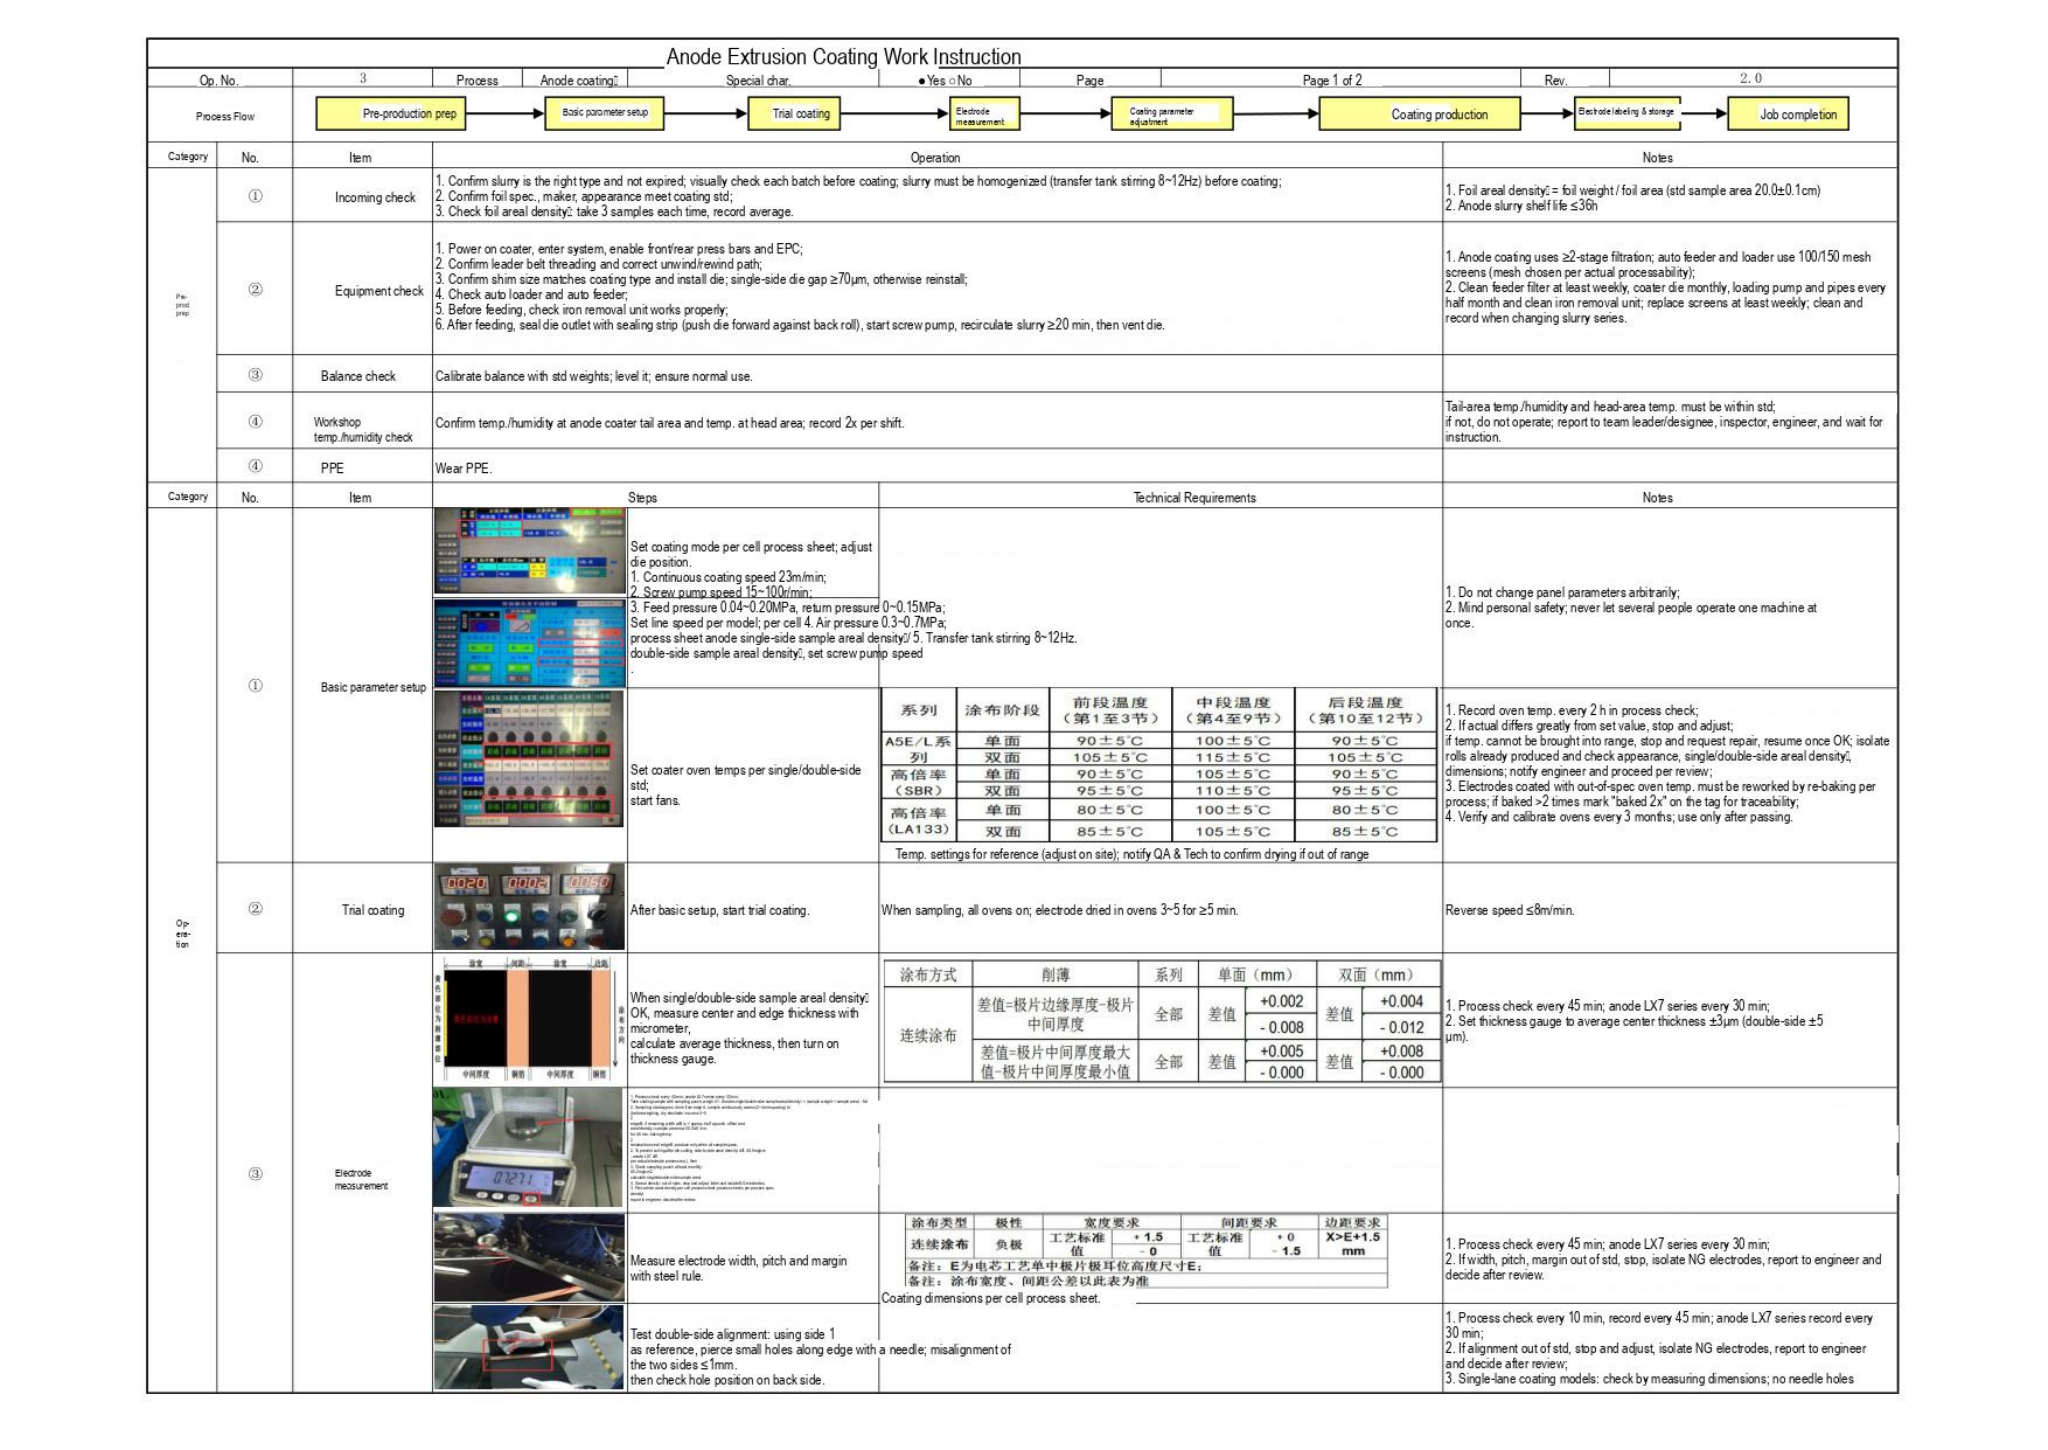Anode Extrusion Coating Work Instruction

| Op. No. | 3 | Process | Anode coating | Special char. | ●Yes ○No | Page | Page 1 of 2 | Rev. | 2.0 |
|---|---|---|---|---|---|---|---|---|---|

Process Flow: Pre-production prep → Basic parameter setup → Trial coating → Electrode measurement → Coating parameter adjustment → Coating production → Electrode labeling & storage → Job completion

| Category | No. | Item | Operation | Notes |
|---|---|---|---|---|
| Pre-prod prep | ① | Incoming check | 1. Confirm slurry is the right type and not expired; visually check each batch before coating; slurry must be homogenized (transfer tank stirring 8~12Hz) before coating;<br>2. Confirm foil spec., maker, appearance meet coating std;<br>3. Check foil areal density: take 3 samples each time, record average. | 1. Foil areal density = foil weight / foil area (std sample area 20.0±0.1cm)<br>2. Anode slurry shelf life ≤36h |
| | ② | Equipment check | 1. Power on coater, enter system, enable front/rear press bars and EPC;<br>2. Confirm leader belt threading and correct unwind/rewind path;<br>3. Confirm shim size matches coating type and install die; single-side die gap ≥70μm, otherwise reinstall;<br>4. Check auto loader and auto feeder;<br>5. Before feeding, check iron removal unit works properly;<br>6. After feeding, seal die outlet with sealing strip (push die forward against back roll), start screw pump, recirculate slurry ≥20 min, then vent die. | 1. Anode coating uses ≥2-stage filtration; auto feeder and loader use 100/150 mesh screens (mesh chosen per actual processability);<br>2. Clean feeder filter at least weekly, coater die monthly, loading pump and pipes every half month and clean iron removal unit; replace screens at least weekly; clean and record when changing slurry series. |
| | ③ | Balance check | Calibrate balance with std weights; level it; ensure normal use. | |
| | ④ | Workshop temp./humidity check | Confirm temp./humidity at anode coater tail area and temp. at head area; record 2x per shift. | Tail-area temp./humidity and head-area temp. must be within std; if not, do not operate; report to team leader/designee, inspector, engineer, and wait for instruction. |
| | ④ | PPE | Wear PPE. | |

| Category | No. | Item | Steps | Technical Requirements | Notes |
|---|---|---|---|---|---|
| Operation | ① | Basic parameter setup | Set coating mode per cell process sheet; adjust die position.<br>1. Continuous coating speed 23m/min;<br>2. Screw pump speed 15~100r/min;<br>3. Feed pressure 0.04~0.20MPa, return pressure 0~0.15MPa;<br>Set line speed per model; per cell 4. Air pressure 0.3~0.7MPa;<br>process sheet anode single-side sample areal density/ 5. Transfer tank stirring 8~12Hz.<br>double-side sample areal density, set screw pump speed | | 1. Do not change panel parameters arbitrarily;<br>2. Mind personal safety; never let several people operate one machine at once. |
| | | | Set coater oven temps per single/double-side std;<br>start fans. | (see oven temperature table below)<br>Temp. settings for reference (adjust on site); notify QA & Tech to confirm drying if out of range | 1. Record oven temp. every 2 h in process check;<br>2. If actual differs greatly from set value, stop and adjust;<br>if temp. cannot be brought into range, stop and request repair, resume once OK; isolate rolls already produced and check appearance, single/double-side areal density, dimensions; notify engineer and proceed per review;<br>3. Electrodes coated with out-of-spec oven temp. must be reworked by re-baking per process; if baked >2 times mark "baked 2x" on the tag for traceability;<br>4. Verify and calibrate ovens every 3 months; use only after passing. |
| | ② | Trial coating | After basic setup, start trial coating. | When sampling, all ovens on; electrode dried in ovens 3~5 for ≥5 min. | Reverse speed ≤8m/min. |
| | ③ | Electrode measurement | When single/double-side sample areal density OK, measure center and edge thickness with micrometer,<br>calculate average thickness, then turn on thickness gauge. | (see thinning table below) | 1. Process check every 45 min; anode LX7 series every 30 min;<br>2. Set thickness gauge to average center thickness ±3μm (double-side ±5 μm). |
| | | | Measure electrode width, pitch and margin with steel rule. | (see dimension table below)<br>Coating dimensions per cell process sheet. | 1. Process check every 45 min; anode LX7 series every 30 min;<br>2. If width, pitch, margin out of std, stop, isolate NG electrodes, report to engineer and decide after review. |
| | | | Test double-side alignment: using side 1 as reference, pierce small holes along edge with a needle; misalignment of the two sides ≤1mm.<br>then check hole position on back side. | | 1. Process check every 10 min, record every 45 min; anode LX7 series record every 30 min;<br>2. If alignment out of std, stop and adjust, isolate NG electrodes, report to engineer and decide after review;<br>3. Single-lane coating models: check by measuring dimensions; no needle holes |

Oven temperature table:

| 系列 | 涂布阶段 | 前段温度（第1至3节） | 中段温度（第4至9节） | 后段温度（第10至12节） |
|---|---|---|---|---|
| A5E/L系列 | 单面 | 90±5℃ | 100±5℃ | 90±5℃ |
| | 双面 | 105±5℃ | 115±5℃ | 105±5℃ |
| 高倍率（SBR） | 单面 | 90±5℃ | 105±5℃ | 90±5℃ |
| | 双面 | 95±5℃ | 110±5℃ | 95±5℃ |
| 高倍率（LA133） | 单面 | 80±5℃ | 100±5℃ | 80±5℃ |
| | 双面 | 85±5℃ | 105±5℃ | 85±5℃ |

Thinning table:

| 涂布方式 | 削薄 | 系列 | 单面（mm） | | 双面（mm） | |
|---|---|---|---|---|---|---|
| 连续涂布 | 差值=极片边缘厚度-极片中间厚度 | 全部 | 差值 | +0.002 / -0.008 | 差值 | +0.004 / -0.012 |
| | 差值=极片中间厚度最大值-极片中间厚度最小值 | 全部 | 差值 | +0.005 / -0.000 | 差值 | +0.008 / -0.000 |

Dimension table:

| 涂布类型 | 极性 | 宽度要求 | | 间距要求 | | 边距要求 |
|---|---|---|---|---|---|---|
| 连续涂布 | 负极 | 工艺标准值 | +1.5 / -0 | 工艺标准值 | +0 / -1.5 | X>E+1.5 mm |

备注：E为电芯工艺单中极片极耳位高度尺寸E;
备注：涂布宽度、间距公差以此表为准

Words in photographs (thickness diagram): 中间厚度, 铜箔, 中间厚度, 铜箔
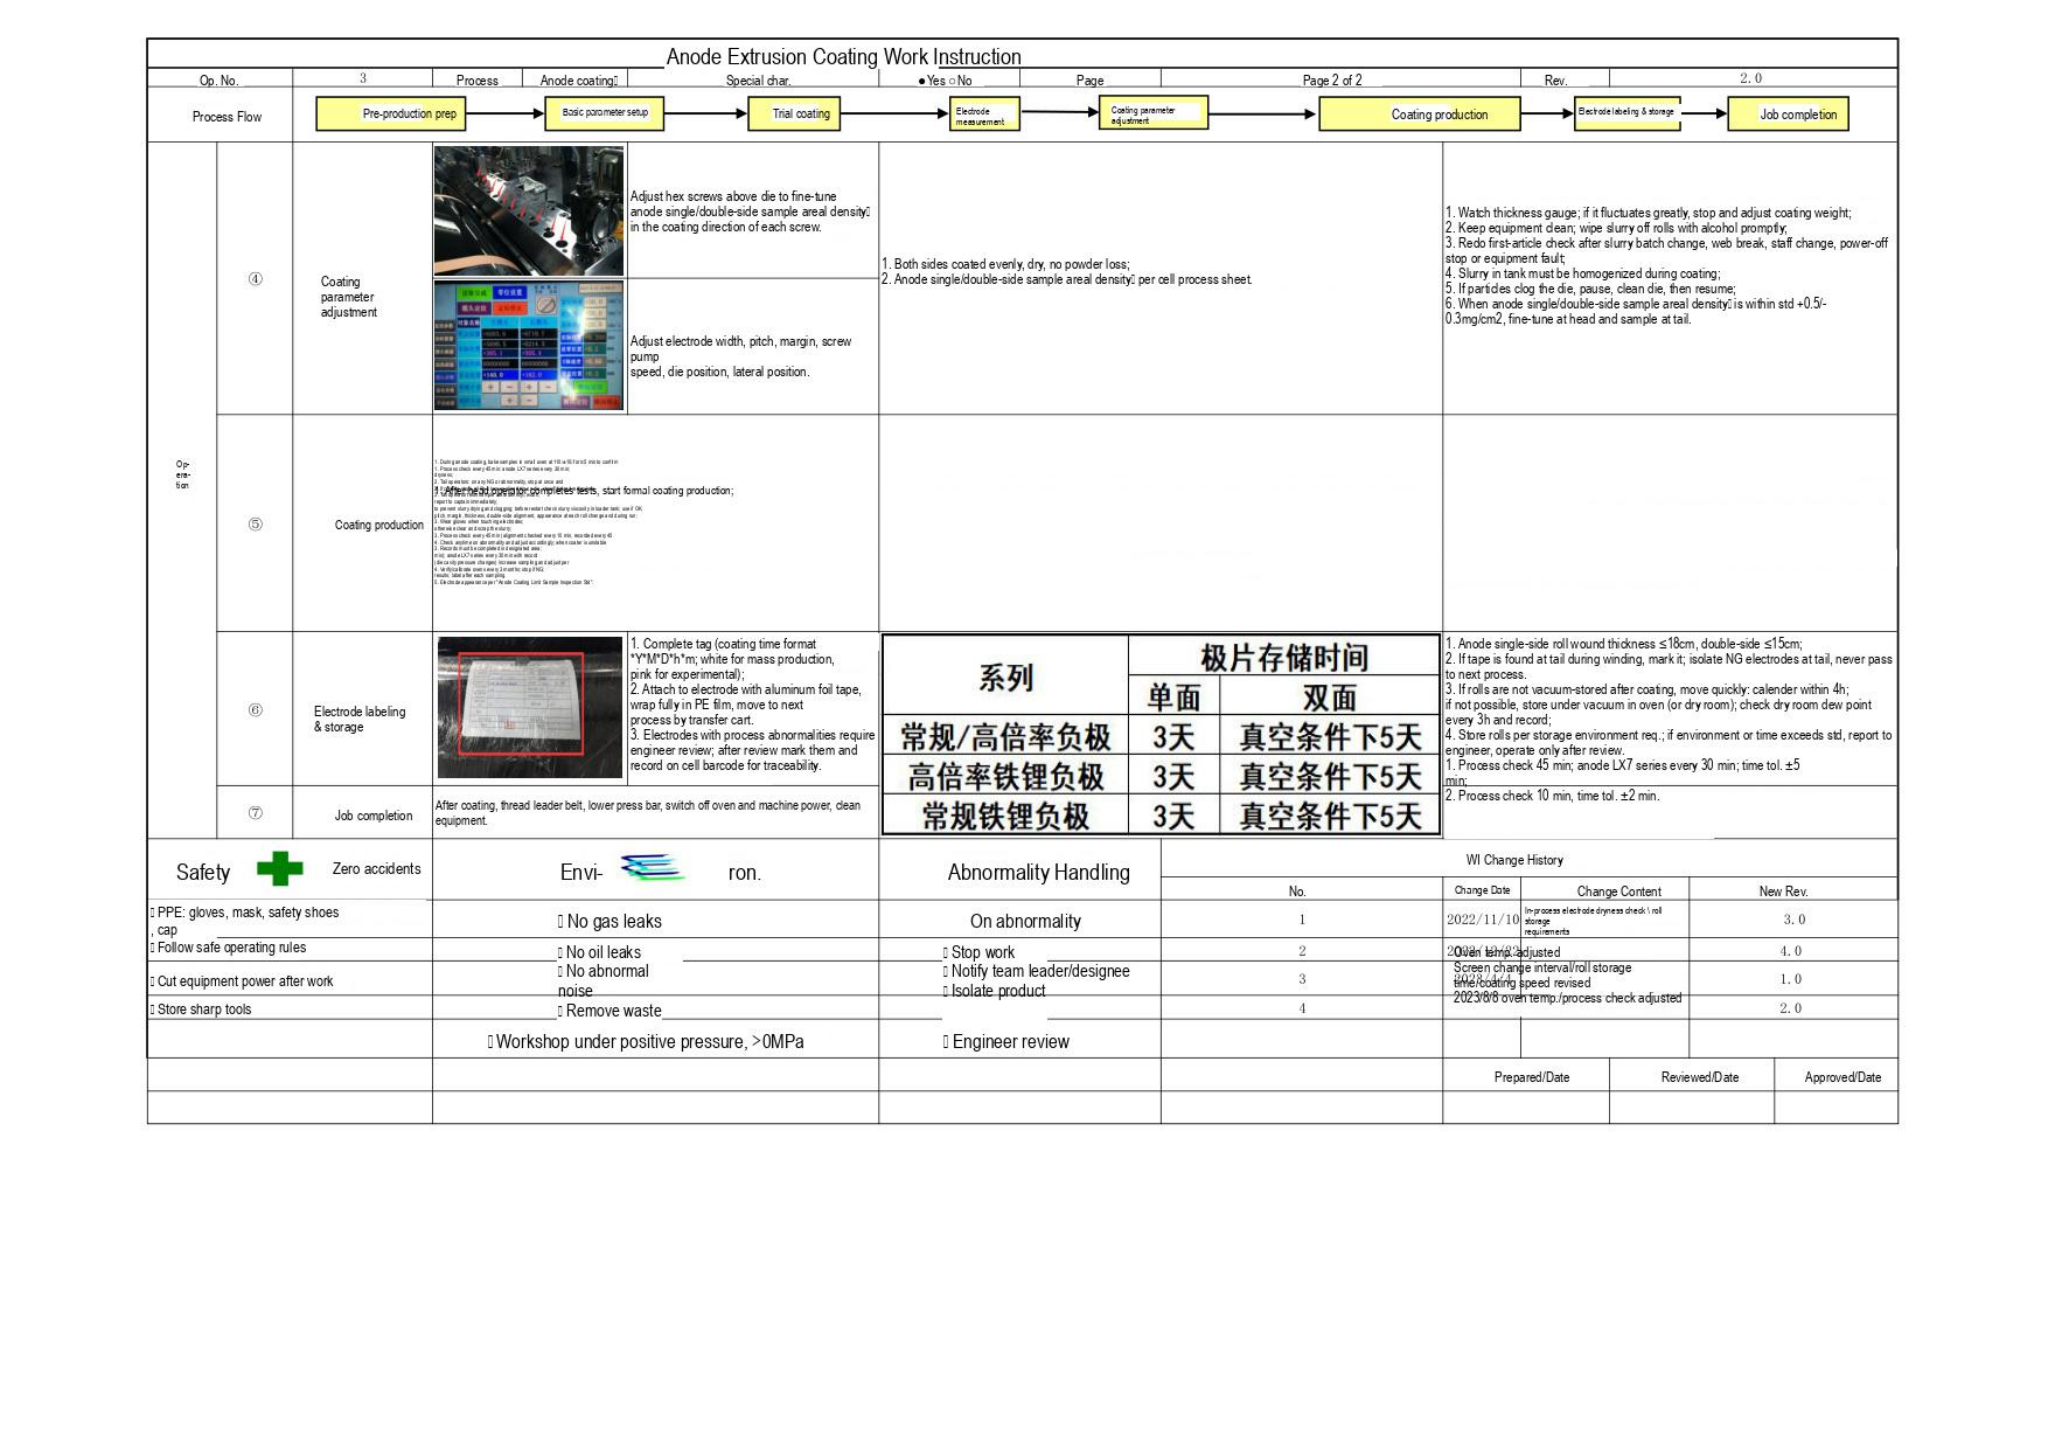# Anode Extrusion Coating Work Instruction

| Op. No. | 3 | Process | Anode coating | Special char. | ●Yes ○No | Page | Page 2 of 2 | Rev. | 2.0 |
|---|---|---|---|---|---|---|---|---|---|

Process Flow: Pre-production prep → Basic parameter setup → Trial coating → Electrode measurement → Coating parameter adjustment → Coating production → Electrode labeling & storage → Job completion

Op-era-tion

| | | | | |
|---|---|---|---|---|
| ④ | Coating parameter adjustment | Adjust hex screws above die to fine-tune anode single/double-side sample areal density in the coating direction of each screw.<br>Adjust electrode width, pitch, margin, screw pump speed, die position, lateral position. | 1. Both sides coated evenly, dry, no powder loss;<br>2. Anode single/double-side sample areal density per cell process sheet | 1. Watch thickness gauge; if it fluctuates greatly, stop and adjust coating weight;<br>2. Keep equipment clean; wipe slurry off rolls with alcohol promptly;<br>3. Redo first-article check after slurry batch change, web break, staff change, power-off stop or equipment fault;<br>4. Slurry in tank must be homogenized during coating;<br>5. If particles clog the die, pause, clean die, then resume;<br>6. When anode single/double-side sample areal density is within std +0.5/-0.3mg/cm2, fine-tune at head and sample at tail. |
| ⑤ | Coating production | 1. After head operator completes tests, start formal coating production; | | |
| ⑥ | Electrode labeling & storage | 1. Complete tag (coating time format *Y*M*D*h*m; white for mass production, pink for experimental);<br>2. Attach to electrode with aluminum foil tape, wrap fully in PE film, move to next process by transfer cart.<br>3. Electrodes with process abnormalities require engineer review; after review mark them and record on cell barcode for traceability. | (see table below) | 1. Anode single-side roll wound thickness ≤18cm, double-side ≤15cm;<br>2. If tape is found at tail during winding, mark it; isolate NG electrodes at tail, never pass to next process.<br>3. If rolls are not vacuum-stored after coating, move quickly: calender within 4h; if not possible, store under vacuum in oven (or dry room); check dry room dew point every 3h and record;<br>4. Store rolls per storage environment req.; if environment or time exceeds std, report to engineer, operate only after review.<br>1. Process check 45 min; anode LX7 series every 30 min; time tol. ±5 min;<br>2. Process check 10 min, time tol. ±2 min. |
| ⑦ | Job completion | After coating, thread leader belt, lower press bar, switch off oven and machine power, clean equipment. | | |

| 系列 | 极片存储时间 单面 | 极片存储时间 双面 |
|---|---|---|
| 常规/高倍率负极 | 3天 | 真空条件下5天 |
| 高倍率铁锂负极 | 3天 | 真空条件下5天 |
| 常规铁锂负极 | 3天 | 真空条件下5天 |

| Safety — Zero accidents | Envi- ron. | Abnormality Handling |
|---|---|---|
| PPE: gloves, mask, safety shoes, cap | No gas leaks | On abnormality |
| Follow safe operating rules | No oil leaks | Stop work |
| Cut equipment power after work | No abnormal noise | Notify team leader/designee |
| Store sharp tools | Remove waste | Isolate product |
| | Workshop under positive pressure, >0MPa | Engineer review |

WI Change History

| No. | Change Date | Change Content | New Rev. |
|---|---|---|---|
| 1 | 2022/11/10 | In-process electrode dryness check\roll storage requirements | 3.0 |
| 2 | | Oven temp. adjusted | 4.0 |
| 3 | | Screen change interval/roll storage time/coating speed revised | 1.0 |
| 4 | | 2023/8/8 oven temp./process check adjusted | 2.0 |

| Prepared/Date | Reviewed/Date | Approved/Date |
|---|---|---|
| | | |